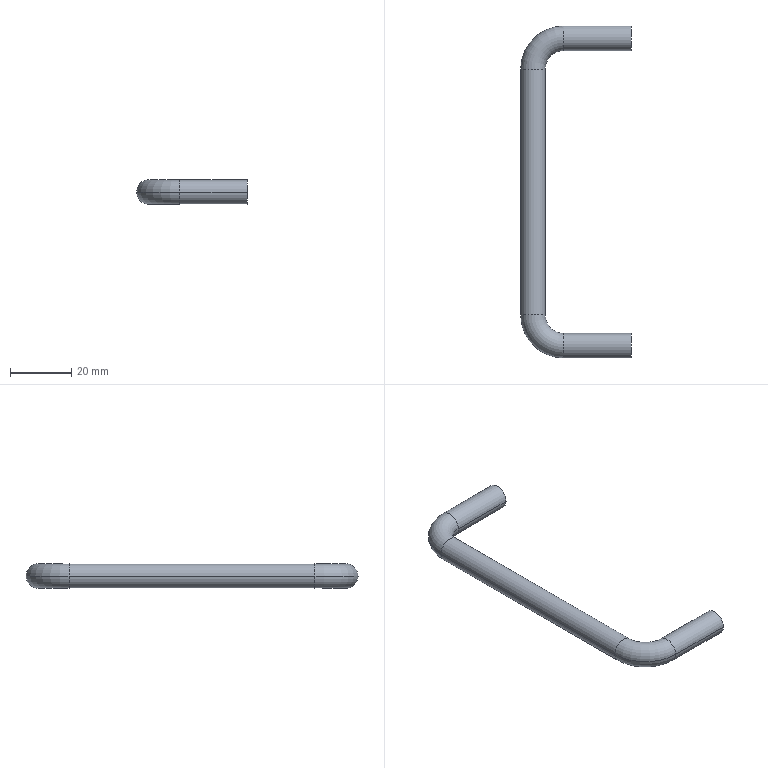Part | SolidWorks | features BaseBody 1 | 1 solid | 18 faces | box 36 x 108 x 8 mm | volume 7468 mm3 | cylinder 10 | torus 4 | plane 4 | commonest cylinder face diameters 8 x6 4.2 x4
STEP:
#1=CARTESIAN_POINT('',(-4.,-40.,0.));
#2=VERTEX_POINT('',#1);
#3=CARTESIAN_POINT('',(4.,-40.,0.));
#4=VERTEX_POINT('',#3);
#5=CARTESIAN_POINT('',(0.,-40.,0.));
#6=DIRECTION('',(0.,1.,0.));
#7=DIRECTION('',(1.,0.,0.));
#8=AXIS2_PLACEMENT_3D('',#5,#6,#7);
#9=CIRCLE('',#8,4.);
#10=EDGE_CURVE('',#2,#4,#9,.T.);
#11=ORIENTED_EDGE('',*,*,#10,.F.);
#12=CARTESIAN_POINT('',(10.,-54.,0.));
#13=VERTEX_POINT('',#12);
#14=CARTESIAN_POINT('',(10.,-40.,0.));
#15=DIRECTION('',(0.,0.,1.));
#16=DIRECTION('',(1.,0.,0.));
#17=AXIS2_PLACEMENT_3D('',#14,#15,#16);
#18=CIRCLE('',#17,14.);
#19=EDGE_CURVE('',#2,#13,#18,.T.);
#20=ORIENTED_EDGE('',*,*,#19,.T.);
#21=CARTESIAN_POINT('',(10.,-46.,0.));
#22=VERTEX_POINT('',#21);
#23=CARTESIAN_POINT('',(10.,-50.,0.));
#24=DIRECTION('',(-1.,0.,0.));
#25=DIRECTION('',(0.,-1.,0.));
#26=AXIS2_PLACEMENT_3D('',#23,#24,#25);
#27=CIRCLE('',#26,4.);
#28=EDGE_CURVE('',#13,#22,#27,.T.);
#29=ORIENTED_EDGE('',*,*,#28,.T.);
#30=CARTESIAN_POINT('',(10.,-40.,0.));
#31=DIRECTION('',(0.,0.,1.));
#32=DIRECTION('',(1.,0.,0.));
#33=AXIS2_PLACEMENT_3D('',#30,#31,#32);
#34=CIRCLE('',#33,6.);
#35=EDGE_CURVE('',#4,#22,#34,.T.);
#36=ORIENTED_EDGE('',*,*,#35,.F.);
#37=EDGE_LOOP('',(#11,#20,#29,#36));
#38=FACE_OUTER_BOUND('',#37,.T.);
#39=CARTESIAN_POINT('',(10.,-40.,0.));
#40=DIRECTION('',(0.,0.,1.));
#41=DIRECTION('',(1.,0.,0.));
#42=AXIS2_PLACEMENT_3D('',#39,#40,#41);
#43=TOROIDAL_SURFACE('',#42,10.,4.);
#44=ADVANCED_FACE('',(#38),#43,.T.);
#45=CARTESIAN_POINT('',(10.,46.,0.));
#46=VERTEX_POINT('',#45);
#47=CARTESIAN_POINT('',(10.,54.,0.));
#48=VERTEX_POINT('',#47);
#49=CARTESIAN_POINT('',(10.,50.,0.));
#50=DIRECTION('',(-1.,0.,0.));
#51=DIRECTION('',(0.,1.,0.));
#52=AXIS2_PLACEMENT_3D('',#49,#50,#51);
#53=CIRCLE('',#52,4.);
#54=EDGE_CURVE('',#46,#48,#53,.T.);
#55=ORIENTED_EDGE('',*,*,#54,.T.);
#56=CARTESIAN_POINT('',(-4.,40.,0.));
#57=VERTEX_POINT('',#56);
#58=CARTESIAN_POINT('',(10.,40.,0.));
#59=DIRECTION('',(0.,0.,1.));
#60=DIRECTION('',(1.,0.,0.));
#61=AXIS2_PLACEMENT_3D('',#58,#59,#60);
#62=CIRCLE('',#61,14.);
#63=EDGE_CURVE('',#48,#57,#62,.T.);
#64=ORIENTED_EDGE('',*,*,#63,.T.);
#65=CARTESIAN_POINT('',(4.,40.,0.));
#66=VERTEX_POINT('',#65);
#67=CARTESIAN_POINT('',(0.,40.,0.));
#68=DIRECTION('',(0.,-1.,0.));
#69=DIRECTION('',(1.,0.,0.));
#70=AXIS2_PLACEMENT_3D('',#67,#68,#69);
#71=CIRCLE('',#70,4.);
#72=EDGE_CURVE('',#66,#57,#71,.T.);
#73=ORIENTED_EDGE('',*,*,#72,.F.);
#74=CARTESIAN_POINT('',(10.,40.,0.));
#75=DIRECTION('',(0.,0.,1.));
#76=DIRECTION('',(1.,0.,0.));
#77=AXIS2_PLACEMENT_3D('',#74,#75,#76);
#78=CIRCLE('',#77,6.);
#79=EDGE_CURVE('',#46,#66,#78,.T.);
#80=ORIENTED_EDGE('',*,*,#79,.F.);
#81=EDGE_LOOP('',(#55,#64,#73,#80));
#82=FACE_OUTER_BOUND('',#81,.T.);
#83=CARTESIAN_POINT('',(10.,40.,0.));
#84=DIRECTION('',(0.,0.,1.));
#85=DIRECTION('',(1.,0.,0.));
#86=AXIS2_PLACEMENT_3D('',#83,#84,#85);
#87=TOROIDAL_SURFACE('',#86,10.,4.);
#88=ADVANCED_FACE('',(#82),#87,.T.);
#89=ORIENTED_EDGE('',*,*,#72,.T.);
#90=CARTESIAN_POINT('',(-4.,40.,0.));
#91=DIRECTION('',(0.,-1.,0.));
#92=VECTOR('',#91,1000.);
#93=LINE('',#90,#92);
#94=EDGE_CURVE('',#57,#2,#93,.T.);
#95=ORIENTED_EDGE('',*,*,#94,.T.);
#96=ORIENTED_EDGE('',*,*,#10,.T.);
#97=CARTESIAN_POINT('',(4.,40.,0.));
#98=DIRECTION('',(0.,-1.,0.));
#99=VECTOR('',#98,1000.);
#100=LINE('',#97,#99);
#101=EDGE_CURVE('',#66,#4,#100,.T.);
#102=ORIENTED_EDGE('',*,*,#101,.F.);
#103=EDGE_LOOP('',(#89,#95,#96,#102));
#104=FACE_OUTER_BOUND('',#103,.T.);
#105=CARTESIAN_POINT('',(0.,40.,0.));
#106=DIRECTION('',(0.,-1.,0.));
#107=DIRECTION('',(1.,0.,0.));
#108=AXIS2_PLACEMENT_3D('',#105,#106,#107);
#109=CYLINDRICAL_SURFACE('',#108,4.);
#110=ADVANCED_FACE('',(#104),#109,.T.);
#111=ORIENTED_EDGE('',*,*,#28,.F.);
#112=CARTESIAN_POINT('',(32.,-54.,0.));
#113=VERTEX_POINT('',#112);
#114=CARTESIAN_POINT('',(10.,-54.,0.));
#115=DIRECTION('',(1.,0.,0.));
#116=VECTOR('',#115,1000.);
#117=LINE('',#114,#116);
#118=EDGE_CURVE('',#13,#113,#117,.T.);
#119=ORIENTED_EDGE('',*,*,#118,.T.);
#120=CARTESIAN_POINT('',(32.,-46.,0.));
#121=VERTEX_POINT('',#120);
#122=CARTESIAN_POINT('',(32.,-50.,0.));
#123=DIRECTION('',(-1.,0.,0.));
#124=DIRECTION('',(0.,1.,0.));
#125=AXIS2_PLACEMENT_3D('',#122,#123,#124);
#126=CIRCLE('',#125,4.);
#127=EDGE_CURVE('',#113,#121,#126,.T.);
#128=ORIENTED_EDGE('',*,*,#127,.T.);
#129=CARTESIAN_POINT('',(10.,-46.,0.));
#130=DIRECTION('',(1.,0.,0.));
#131=VECTOR('',#130,1000.);
#132=LINE('',#129,#131);
#133=EDGE_CURVE('',#22,#121,#132,.T.);
#134=ORIENTED_EDGE('',*,*,#133,.F.);
#135=EDGE_LOOP('',(#111,#119,#128,#134));
#136=FACE_OUTER_BOUND('',#135,.T.);
#137=CARTESIAN_POINT('',(10.,-50.,0.));
#138=DIRECTION('',(1.,0.,0.));
#139=DIRECTION('',(0.,1.,0.));
#140=AXIS2_PLACEMENT_3D('',#137,#138,#139);
#141=CYLINDRICAL_SURFACE('',#140,4.);
#142=ADVANCED_FACE('',(#136),#141,.T.);
#143=ORIENTED_EDGE('',*,*,#54,.F.);
#144=CARTESIAN_POINT('',(32.,46.,0.));
#145=VERTEX_POINT('',#144);
#146=CARTESIAN_POINT('',(10.,46.,0.));
#147=DIRECTION('',(1.,0.,0.));
#148=VECTOR('',#147,1000.);
#149=LINE('',#146,#148);
#150=EDGE_CURVE('',#46,#145,#149,.T.);
#151=ORIENTED_EDGE('',*,*,#150,.T.);
#152=CARTESIAN_POINT('',(32.,54.,0.));
#153=VERTEX_POINT('',#152);
#154=CARTESIAN_POINT('',(32.,50.,0.));
#155=DIRECTION('',(-1.,0.,0.));
#156=DIRECTION('',(0.,1.,0.));
#157=AXIS2_PLACEMENT_3D('',#154,#155,#156);
#158=CIRCLE('',#157,4.);
#159=EDGE_CURVE('',#145,#153,#158,.T.);
#160=ORIENTED_EDGE('',*,*,#159,.T.);
#161=CARTESIAN_POINT('',(10.,54.,0.));
#162=DIRECTION('',(1.,0.,0.));
#163=VECTOR('',#162,1000.);
#164=LINE('',#161,#163);
#165=EDGE_CURVE('',#48,#153,#164,.T.);
#166=ORIENTED_EDGE('',*,*,#165,.F.);
#167=EDGE_LOOP('',(#143,#151,#160,#166));
#168=FACE_OUTER_BOUND('',#167,.T.);
#169=CARTESIAN_POINT('',(10.,50.,0.));
#170=DIRECTION('',(1.,0.,0.));
#171=DIRECTION('',(0.,1.,0.));
#172=AXIS2_PLACEMENT_3D('',#169,#170,#171);
#173=CYLINDRICAL_SURFACE('',#172,4.);
#174=ADVANCED_FACE('',(#168),#173,.T.);
#175=CARTESIAN_POINT('',(19.6,-50.,2.1));
#176=VERTEX_POINT('',#175);
#177=CARTESIAN_POINT('',(19.6,-50.,-2.1));
#178=VERTEX_POINT('',#177);
#179=CARTESIAN_POINT('',(19.6,-50.,0.));
#180=DIRECTION('',(1.,0.,0.));
#181=DIRECTION('',(0.,0.,-1.));
#182=AXIS2_PLACEMENT_3D('',#179,#180,#181);
#183=CIRCLE('',#182,2.1);
#184=EDGE_CURVE('',#176,#178,#183,.T.);
#185=ORIENTED_EDGE('',*,*,#184,.F.);
#186=CARTESIAN_POINT('',(32.,-50.,2.1));
#187=VERTEX_POINT('',#186);
#188=CARTESIAN_POINT('',(32.,-50.,2.1));
#189=DIRECTION('',(1.,0.,0.));
#190=VECTOR('',#189,1000.);
#191=LINE('',#188,#190);
#192=EDGE_CURVE('',#176,#187,#191,.T.);
#193=ORIENTED_EDGE('',*,*,#192,.T.);
#194=CARTESIAN_POINT('',(32.,-50.,-2.1));
#195=VERTEX_POINT('',#194);
#196=CARTESIAN_POINT('',(32.,-50.,0.));
#197=DIRECTION('',(-1.,0.,0.));
#198=DIRECTION('',(0.,0.,-1.));
#199=AXIS2_PLACEMENT_3D('',#196,#197,#198);
#200=CIRCLE('',#199,2.1);
#201=EDGE_CURVE('',#195,#187,#200,.T.);
#202=ORIENTED_EDGE('',*,*,#201,.F.);
#203=CARTESIAN_POINT('',(32.,-50.,-2.1));
#204=DIRECTION('',(1.,0.,0.));
#205=VECTOR('',#204,1000.);
#206=LINE('',#203,#205);
#207=EDGE_CURVE('',#178,#195,#206,.T.);
#208=ORIENTED_EDGE('',*,*,#207,.F.);
#209=EDGE_LOOP('',(#185,#193,#202,#208));
#210=FACE_OUTER_BOUND('',#209,.T.);
#211=CARTESIAN_POINT('',(32.,-50.,0.));
#212=DIRECTION('',(1.,0.,0.));
#213=DIRECTION('',(0.,0.,-1.));
#214=AXIS2_PLACEMENT_3D('',#211,#212,#213);
#215=CYLINDRICAL_SURFACE('',#214,2.1);
#216=ADVANCED_FACE('',(#210),#215,.F.);
#217=CARTESIAN_POINT('',(19.6,50.,2.1));
#218=VERTEX_POINT('',#217);
#219=CARTESIAN_POINT('',(19.6,50.,-2.1));
#220=VERTEX_POINT('',#219);
#221=CARTESIAN_POINT('',(19.6,50.,0.));
#222=DIRECTION('',(1.,0.,0.));
#223=DIRECTION('',(0.,0.,-1.));
#224=AXIS2_PLACEMENT_3D('',#221,#222,#223);
#225=CIRCLE('',#224,2.1);
#226=EDGE_CURVE('',#218,#220,#225,.T.);
#227=ORIENTED_EDGE('',*,*,#226,.F.);
#228=CARTESIAN_POINT('',(32.,50.,2.1));
#229=VERTEX_POINT('',#228);
#230=CARTESIAN_POINT('',(32.,50.,2.1));
#231=DIRECTION('',(1.,0.,0.));
#232=VECTOR('',#231,1000.);
#233=LINE('',#230,#232);
#234=EDGE_CURVE('',#218,#229,#233,.T.);
#235=ORIENTED_EDGE('',*,*,#234,.T.);
#236=CARTESIAN_POINT('',(32.,50.,-2.1));
#237=VERTEX_POINT('',#236);
#238=CARTESIAN_POINT('',(32.,50.,0.));
#239=DIRECTION('',(1.,0.,0.));
#240=DIRECTION('',(0.,0.,-1.));
#241=AXIS2_PLACEMENT_3D('',#238,#239,#240);
#242=CIRCLE('',#241,2.1);
#243=EDGE_CURVE('',#229,#237,#242,.T.);
#244=ORIENTED_EDGE('',*,*,#243,.T.);
#245=CARTESIAN_POINT('',(32.,50.,-2.1));
#246=DIRECTION('',(1.,0.,0.));
#247=VECTOR('',#246,1000.);
#248=LINE('',#245,#247);
#249=EDGE_CURVE('',#220,#237,#248,.T.);
#250=ORIENTED_EDGE('',*,*,#249,.F.);
#251=EDGE_LOOP('',(#227,#235,#244,#250));
#252=FACE_OUTER_BOUND('',#251,.T.);
#253=CARTESIAN_POINT('',(32.,50.,0.));
#254=DIRECTION('',(1.,0.,0.));
#255=DIRECTION('',(0.,0.,-1.));
#256=AXIS2_PLACEMENT_3D('',#253,#254,#255);
#257=CYLINDRICAL_SURFACE('',#256,2.1);
#258=ADVANCED_FACE('',(#252),#257,.F.);
#259=CARTESIAN_POINT('',(19.6,50.,0.));
#260=DIRECTION('',(1.,0.,0.));
#261=DIRECTION('',(0.,0.,-1.));
#262=AXIS2_PLACEMENT_3D('',#259,#260,#261);
#263=CIRCLE('',#262,2.1);
#264=EDGE_CURVE('',#220,#218,#263,.T.);
#265=ORIENTED_EDGE('',*,*,#264,.T.);
#266=ORIENTED_EDGE('',*,*,#226,.T.);
#267=EDGE_LOOP('',(#265,#266));
#268=FACE_OUTER_BOUND('',#267,.T.);
#269=CARTESIAN_POINT('',(19.6,50.,0.));
#270=DIRECTION('',(-1.,0.,0.));
#271=DIRECTION('',(0.,0.,1.));
#272=AXIS2_PLACEMENT_3D('',#269,#270,#271);
#273=PLANE('',#272);
#274=ADVANCED_FACE('',(#268),#273,.F.);
#275=CARTESIAN_POINT('',(19.6,-50.,0.));
#276=DIRECTION('',(1.,0.,0.));
#277=DIRECTION('',(0.,0.,-1.));
#278=AXIS2_PLACEMENT_3D('',#275,#276,#277);
#279=CIRCLE('',#278,2.1);
#280=EDGE_CURVE('',#178,#176,#279,.T.);
#281=ORIENTED_EDGE('',*,*,#280,.T.);
#282=ORIENTED_EDGE('',*,*,#184,.T.);
#283=EDGE_LOOP('',(#281,#282));
#284=FACE_OUTER_BOUND('',#283,.T.);
#285=CARTESIAN_POINT('',(19.6,-50.,0.));
#286=DIRECTION('',(-1.,0.,0.));
#287=DIRECTION('',(0.,0.,1.));
#288=AXIS2_PLACEMENT_3D('',#285,#286,#287);
#289=PLANE('',#288);
#290=ADVANCED_FACE('',(#284),#289,.F.);
#291=CARTESIAN_POINT('',(32.,50.,0.));
#292=DIRECTION('',(1.,0.,0.));
#293=DIRECTION('',(0.,0.,-1.));
#294=AXIS2_PLACEMENT_3D('',#291,#292,#293);
#295=CIRCLE('',#294,2.1);
#296=EDGE_CURVE('',#237,#229,#295,.T.);
#297=ORIENTED_EDGE('',*,*,#296,.F.);
#298=ORIENTED_EDGE('',*,*,#243,.F.);
#299=EDGE_LOOP('',(#297,#298));
#300=FACE_BOUND('',#299,.T.);
#301=CARTESIAN_POINT('',(32.,50.,0.));
#302=DIRECTION('',(-1.,0.,0.));
#303=DIRECTION('',(0.,1.,0.));
#304=AXIS2_PLACEMENT_3D('',#301,#302,#303);
#305=CIRCLE('',#304,4.);
#306=EDGE_CURVE('',#153,#145,#305,.T.);
#307=ORIENTED_EDGE('',*,*,#306,.F.);
#308=ORIENTED_EDGE('',*,*,#159,.F.);
#309=EDGE_LOOP('',(#307,#308));
#310=FACE_OUTER_BOUND('',#309,.T.);
#311=CARTESIAN_POINT('',(32.,50.,0.));
#312=DIRECTION('',(-1.,0.,0.));
#313=DIRECTION('',(0.,1.,0.));
#314=AXIS2_PLACEMENT_3D('',#311,#312,#313);
#315=PLANE('',#314);
#316=ADVANCED_FACE('',(#300,#310),#315,.F.);
#317=ORIENTED_EDGE('',*,*,#201,.T.);
#318=CARTESIAN_POINT('',(32.,-50.,0.));
#319=DIRECTION('',(-1.,0.,0.));
#320=DIRECTION('',(0.,0.,-1.));
#321=AXIS2_PLACEMENT_3D('',#318,#319,#320);
#322=CIRCLE('',#321,2.1);
#323=EDGE_CURVE('',#187,#195,#322,.T.);
#324=ORIENTED_EDGE('',*,*,#323,.T.);
#325=EDGE_LOOP('',(#317,#324));
#326=FACE_BOUND('',#325,.T.);
#327=CARTESIAN_POINT('',(32.,-50.,0.));
#328=DIRECTION('',(-1.,0.,0.));
#329=DIRECTION('',(0.,1.,0.));
#330=AXIS2_PLACEMENT_3D('',#327,#328,#329);
#331=CIRCLE('',#330,4.);
#332=EDGE_CURVE('',#121,#113,#331,.T.);
#333=ORIENTED_EDGE('',*,*,#332,.F.);
#334=ORIENTED_EDGE('',*,*,#127,.F.);
#335=EDGE_LOOP('',(#333,#334));
#336=FACE_OUTER_BOUND('',#335,.T.);
#337=CARTESIAN_POINT('',(32.,-50.,0.));
#338=DIRECTION('',(1.,0.,0.));
#339=DIRECTION('',(0.,1.,0.));
#340=AXIS2_PLACEMENT_3D('',#337,#338,#339);
#341=PLANE('',#340);
#342=ADVANCED_FACE('',(#326,#336),#341,.T.);
#343=ORIENTED_EDGE('',*,*,#234,.F.);
#344=ORIENTED_EDGE('',*,*,#264,.F.);
#345=ORIENTED_EDGE('',*,*,#249,.T.);
#346=ORIENTED_EDGE('',*,*,#296,.T.);
#347=EDGE_LOOP('',(#343,#344,#345,#346));
#348=FACE_OUTER_BOUND('',#347,.T.);
#349=CARTESIAN_POINT('',(32.,50.,0.));
#350=DIRECTION('',(1.,0.,0.));
#351=DIRECTION('',(0.,0.,-1.));
#352=AXIS2_PLACEMENT_3D('',#349,#350,#351);
#353=CYLINDRICAL_SURFACE('',#352,2.1);
#354=ADVANCED_FACE('',(#348),#353,.F.);
#355=ORIENTED_EDGE('',*,*,#192,.F.);
#356=ORIENTED_EDGE('',*,*,#280,.F.);
#357=ORIENTED_EDGE('',*,*,#207,.T.);
#358=ORIENTED_EDGE('',*,*,#323,.F.);
#359=EDGE_LOOP('',(#355,#356,#357,#358));
#360=FACE_OUTER_BOUND('',#359,.T.);
#361=CARTESIAN_POINT('',(32.,-50.,0.));
#362=DIRECTION('',(1.,0.,0.));
#363=DIRECTION('',(0.,0.,-1.));
#364=AXIS2_PLACEMENT_3D('',#361,#362,#363);
#365=CYLINDRICAL_SURFACE('',#364,2.1);
#366=ADVANCED_FACE('',(#360),#365,.F.);
#367=ORIENTED_EDGE('',*,*,#150,.F.);
#368=CARTESIAN_POINT('',(10.,50.,0.));
#369=DIRECTION('',(-1.,0.,0.));
#370=DIRECTION('',(0.,1.,0.));
#371=AXIS2_PLACEMENT_3D('',#368,#369,#370);
#372=CIRCLE('',#371,4.);
#373=EDGE_CURVE('',#48,#46,#372,.T.);
#374=ORIENTED_EDGE('',*,*,#373,.F.);
#375=ORIENTED_EDGE('',*,*,#165,.T.);
#376=ORIENTED_EDGE('',*,*,#306,.T.);
#377=EDGE_LOOP('',(#367,#374,#375,#376));
#378=FACE_OUTER_BOUND('',#377,.T.);
#379=CARTESIAN_POINT('',(10.,50.,0.));
#380=DIRECTION('',(1.,0.,0.));
#381=DIRECTION('',(0.,1.,0.));
#382=AXIS2_PLACEMENT_3D('',#379,#380,#381);
#383=CYLINDRICAL_SURFACE('',#382,4.);
#384=ADVANCED_FACE('',(#378),#383,.T.);
#385=ORIENTED_EDGE('',*,*,#118,.F.);
#386=CARTESIAN_POINT('',(10.,-50.,0.));
#387=DIRECTION('',(-1.,0.,0.));
#388=DIRECTION('',(0.,-1.,0.));
#389=AXIS2_PLACEMENT_3D('',#386,#387,#388);
#390=CIRCLE('',#389,4.);
#391=EDGE_CURVE('',#22,#13,#390,.T.);
#392=ORIENTED_EDGE('',*,*,#391,.F.);
#393=ORIENTED_EDGE('',*,*,#133,.T.);
#394=ORIENTED_EDGE('',*,*,#332,.T.);
#395=EDGE_LOOP('',(#385,#392,#393,#394));
#396=FACE_OUTER_BOUND('',#395,.T.);
#397=CARTESIAN_POINT('',(10.,-50.,0.));
#398=DIRECTION('',(1.,0.,0.));
#399=DIRECTION('',(0.,1.,0.));
#400=AXIS2_PLACEMENT_3D('',#397,#398,#399);
#401=CYLINDRICAL_SURFACE('',#400,4.);
#402=ADVANCED_FACE('',(#396),#401,.T.);
#403=ORIENTED_EDGE('',*,*,#63,.F.);
#404=ORIENTED_EDGE('',*,*,#373,.T.);
#405=ORIENTED_EDGE('',*,*,#79,.T.);
#406=CARTESIAN_POINT('',(0.,40.,0.));
#407=DIRECTION('',(0.,-1.,0.));
#408=DIRECTION('',(1.,0.,0.));
#409=AXIS2_PLACEMENT_3D('',#406,#407,#408);
#410=CIRCLE('',#409,4.);
#411=EDGE_CURVE('',#57,#66,#410,.T.);
#412=ORIENTED_EDGE('',*,*,#411,.F.);
#413=EDGE_LOOP('',(#403,#404,#405,#412));
#414=FACE_OUTER_BOUND('',#413,.T.);
#415=CARTESIAN_POINT('',(10.,40.,0.));
#416=DIRECTION('',(0.,0.,1.));
#417=DIRECTION('',(1.,0.,0.));
#418=AXIS2_PLACEMENT_3D('',#415,#416,#417);
#419=TOROIDAL_SURFACE('',#418,10.,4.);
#420=ADVANCED_FACE('',(#414),#419,.T.);
#421=ORIENTED_EDGE('',*,*,#19,.F.);
#422=CARTESIAN_POINT('',(0.,-40.,0.));
#423=DIRECTION('',(0.,1.,0.));
#424=DIRECTION('',(1.,0.,0.));
#425=AXIS2_PLACEMENT_3D('',#422,#423,#424);
#426=CIRCLE('',#425,4.);
#427=EDGE_CURVE('',#4,#2,#426,.T.);
#428=ORIENTED_EDGE('',*,*,#427,.F.);
#429=ORIENTED_EDGE('',*,*,#35,.T.);
#430=ORIENTED_EDGE('',*,*,#391,.T.);
#431=EDGE_LOOP('',(#421,#428,#429,#430));
#432=FACE_OUTER_BOUND('',#431,.T.);
#433=CARTESIAN_POINT('',(10.,-40.,0.));
#434=DIRECTION('',(0.,0.,1.));
#435=DIRECTION('',(1.,0.,0.));
#436=AXIS2_PLACEMENT_3D('',#433,#434,#435);
#437=TOROIDAL_SURFACE('',#436,10.,4.);
#438=ADVANCED_FACE('',(#432),#437,.T.);
#439=ORIENTED_EDGE('',*,*,#94,.F.);
#440=ORIENTED_EDGE('',*,*,#411,.T.);
#441=ORIENTED_EDGE('',*,*,#101,.T.);
#442=ORIENTED_EDGE('',*,*,#427,.T.);
#443=EDGE_LOOP('',(#439,#440,#441,#442));
#444=FACE_OUTER_BOUND('',#443,.T.);
#445=CARTESIAN_POINT('',(0.,40.,0.));
#446=DIRECTION('',(0.,-1.,0.));
#447=DIRECTION('',(1.,0.,0.));
#448=AXIS2_PLACEMENT_3D('',#445,#446,#447);
#449=CYLINDRICAL_SURFACE('',#448,4.);
#450=ADVANCED_FACE('',(#444),#449,.T.);
#451=CLOSED_SHELL('',(#44,#88,#110,#142,#174,#216,#258,#274,#290,#316,#342,#354,#366,#384,#402,#420,#438,#450));
#452=MANIFOLD_SOLID_BREP('',#451);
#453=CARTESIAN_POINT('',(0.,0.,0.));
#454=DIRECTION('',(0.,0.,1.));
#455=DIRECTION('',(1.,0.,0.));
#456=AXIS2_PLACEMENT_3D('',#453,#454,#455);
#457=(LENGTH_UNIT()NAMED_UNIT(*)SI_UNIT(.MILLI.,.METRE.));
#458=UNCERTAINTY_MEASURE_WITH_UNIT(LENGTH_MEASURE(0.00001),#457,'','');
#459=(NAMED_UNIT(*)PLANE_ANGLE_UNIT()SI_UNIT($,.RADIAN.));
#460=(NAMED_UNIT(*)SI_UNIT($,.STERADIAN.)SOLID_ANGLE_UNIT());
#461=(GEOMETRIC_REPRESENTATION_CONTEXT(3)GLOBAL_UNCERTAINTY_ASSIGNED_CONTEXT((#458))GLOBAL_UNIT_ASSIGNED_CONTEXT((#457,#459,#460))REPRESENTATION_CONTEXT('',''));
#462=ADVANCED_BREP_SHAPE_REPRESENTATION('',(#452,#456),#461);